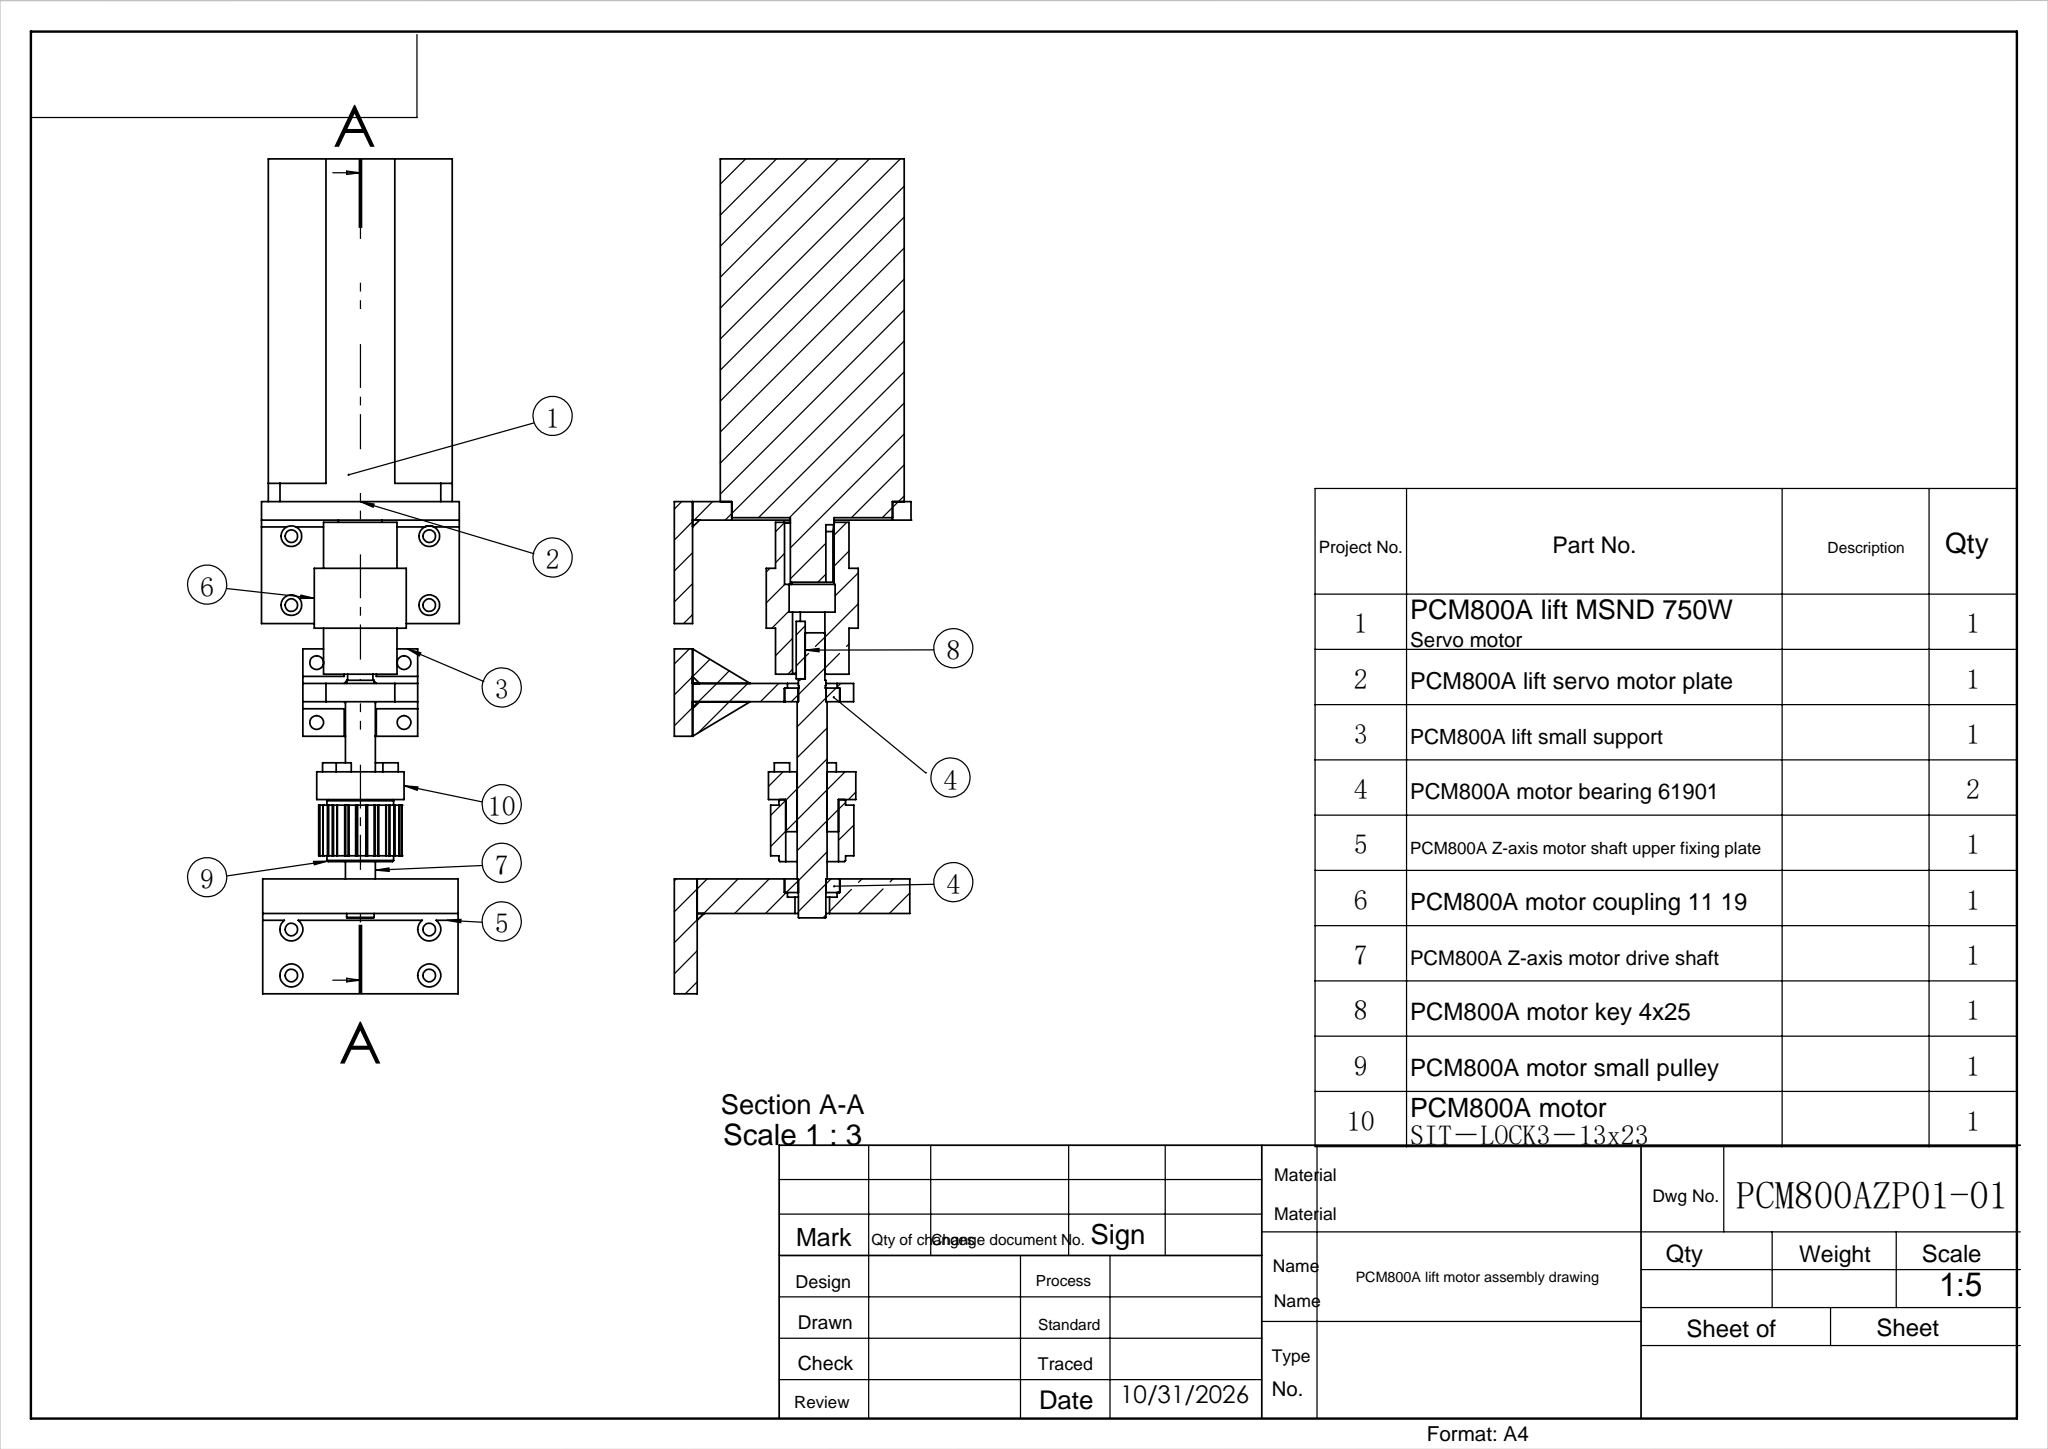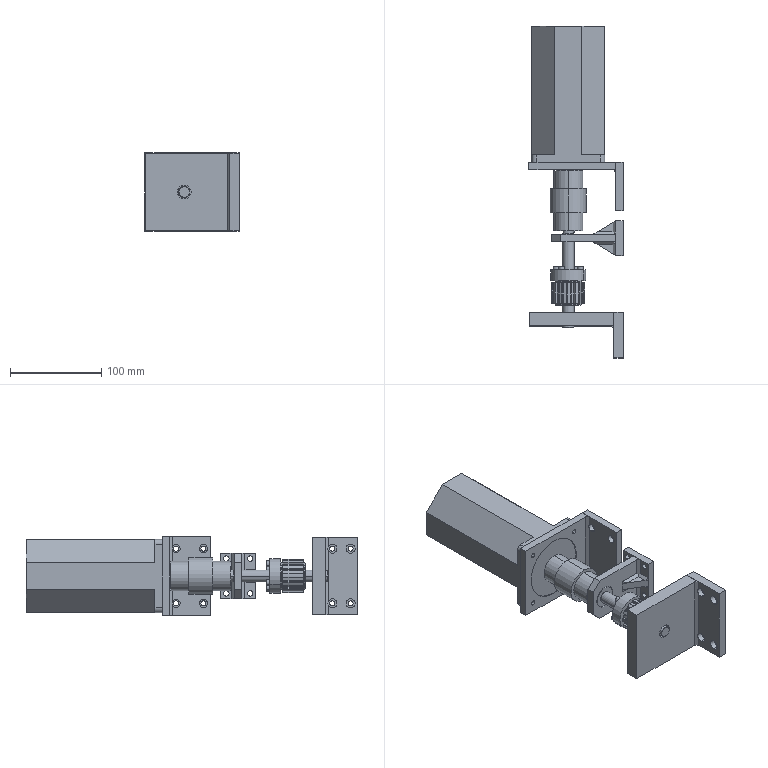Part | SolidWorks | 24 solids | 459 faces | box 103 x 363 x 86 mm | volume 1173870 mm3 | plane 214 | cylinder 208 | cone 31 | torus 6 | commonest cylinder face diameters 0.8 x58 6 x17 5.5 x16 10 x14 36.2 x12 9 x10